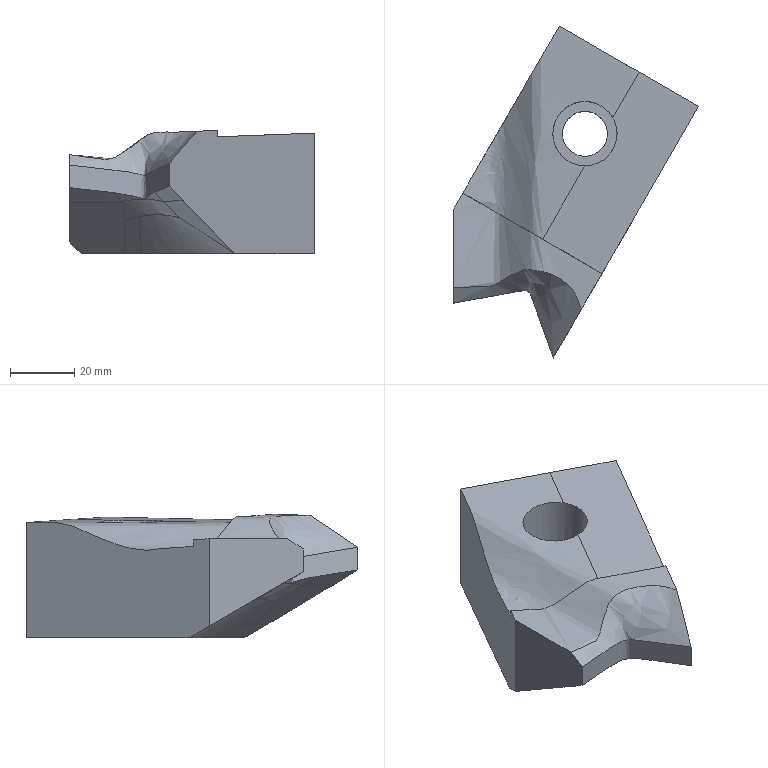Part | NX | features solid 2 | 1 solid | 22 faces | box 76.169 x 103.233 x 38.362 mm | volume 117807 mm3 | spline 13 | plane 7 | cylinder 2 | commonest cylinder face diameters 14 x1 20 x1